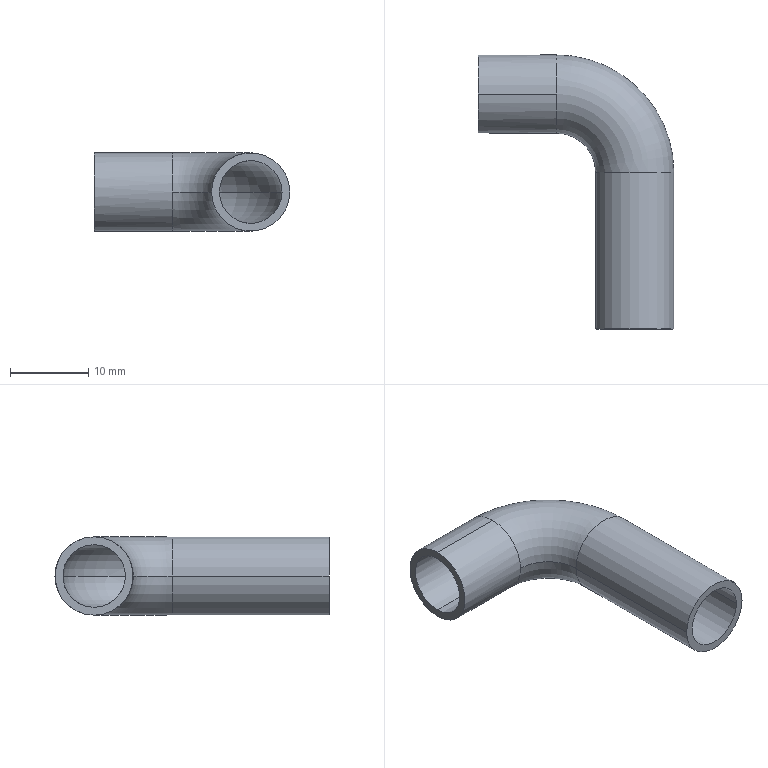Part | SolidWorks | features Sweep 1 | 1 solid | 14 faces | box 25 x 35 x 10 mm | volume 1292 mm3 | cylinder 8 | torus 4 | plane 2 | commonest cylinder face diameters 8 x4 10 x4
STEP:
#1=CARTESIAN_POINT('',(10.,4.,0.));
#2=VERTEX_POINT('',#1);
#3=CARTESIAN_POINT('',(10.,0.,4.));
#4=VERTEX_POINT('',#3);
#5=CARTESIAN_POINT('',(10.,0.,0.));
#6=DIRECTION('',(1.,0.,0.));
#7=DIRECTION('',(0.,0.,-1.));
#8=AXIS2_PLACEMENT_3D('',#5,#6,#7);
#9=CIRCLE('',#8,4.);
#10=EDGE_CURVE('',#2,#4,#9,.T.);
#11=ORIENTED_EDGE('',*,*,#10,.F.);
#12=CARTESIAN_POINT('',(24.,-10.,0.));
#13=VERTEX_POINT('',#12);
#14=CARTESIAN_POINT('',(10.,-10.,0.));
#15=DIRECTION('',(0.,0.,-1.));
#16=DIRECTION('',(-1.,0.,0.));
#17=AXIS2_PLACEMENT_3D('',#14,#15,#16);
#18=CIRCLE('',#17,14.);
#19=EDGE_CURVE('',#2,#13,#18,.T.);
#20=ORIENTED_EDGE('',*,*,#19,.T.);
#21=CARTESIAN_POINT('',(16.,-10.,0.));
#22=VERTEX_POINT('',#21);
#23=CARTESIAN_POINT('',(20.,-10.,0.));
#24=DIRECTION('',(0.,-1.,0.));
#25=DIRECTION('',(0.,0.,-1.));
#26=AXIS2_PLACEMENT_3D('',#23,#24,#25);
#27=CIRCLE('',#26,4.);
#28=EDGE_CURVE('',#13,#22,#27,.T.);
#29=ORIENTED_EDGE('',*,*,#28,.T.);
#30=CARTESIAN_POINT('',(10.,-4.,0.));
#31=VERTEX_POINT('',#30);
#32=CARTESIAN_POINT('',(10.,-10.,0.));
#33=DIRECTION('',(0.,0.,-1.));
#34=DIRECTION('',(-1.,0.,0.));
#35=AXIS2_PLACEMENT_3D('',#32,#33,#34);
#36=CIRCLE('',#35,6.);
#37=EDGE_CURVE('',#31,#22,#36,.T.);
#38=ORIENTED_EDGE('',*,*,#37,.F.);
#39=CARTESIAN_POINT('',(10.,0.,0.));
#40=DIRECTION('',(1.,0.,0.));
#41=DIRECTION('',(0.,0.,-1.));
#42=AXIS2_PLACEMENT_3D('',#39,#40,#41);
#43=CIRCLE('',#42,4.);
#44=EDGE_CURVE('',#4,#31,#43,.T.);
#45=ORIENTED_EDGE('',*,*,#44,.F.);
#46=EDGE_LOOP('',(#11,#20,#29,#38,#45));
#47=FACE_OUTER_BOUND('',#46,.T.);
#48=CARTESIAN_POINT('',(10.,-10.,0.));
#49=DIRECTION('',(0.,0.,-1.));
#50=DIRECTION('',(-1.,0.,0.));
#51=AXIS2_PLACEMENT_3D('',#48,#49,#50);
#52=TOROIDAL_SURFACE('',#51,10.,4.);
#53=ADVANCED_FACE('',(#47),#52,.F.);
#54=CARTESIAN_POINT('',(10.,0.,-5.));
#55=VERTEX_POINT('',#54);
#56=CARTESIAN_POINT('',(10.,5.,0.));
#57=VERTEX_POINT('',#56);
#58=CARTESIAN_POINT('',(10.,0.,0.));
#59=DIRECTION('',(1.,0.,0.));
#60=DIRECTION('',(0.,0.,-1.));
#61=AXIS2_PLACEMENT_3D('',#58,#59,#60);
#62=CIRCLE('',#61,5.);
#63=EDGE_CURVE('',#55,#57,#62,.T.);
#64=ORIENTED_EDGE('',*,*,#63,.T.);
#65=CARTESIAN_POINT('',(25.,-10.,0.));
#66=VERTEX_POINT('',#65);
#67=CARTESIAN_POINT('',(10.,-10.,0.));
#68=DIRECTION('',(0.,0.,-1.));
#69=DIRECTION('',(-1.,0.,0.));
#70=AXIS2_PLACEMENT_3D('',#67,#68,#69);
#71=CIRCLE('',#70,15.);
#72=EDGE_CURVE('',#57,#66,#71,.T.);
#73=ORIENTED_EDGE('',*,*,#72,.T.);
#74=CARTESIAN_POINT('',(15.,-10.,0.));
#75=VERTEX_POINT('',#74);
#76=CARTESIAN_POINT('',(20.,-10.,0.));
#77=DIRECTION('',(0.,-1.,0.));
#78=DIRECTION('',(0.,0.,-1.));
#79=AXIS2_PLACEMENT_3D('',#76,#77,#78);
#80=CIRCLE('',#79,5.);
#81=EDGE_CURVE('',#75,#66,#80,.T.);
#82=ORIENTED_EDGE('',*,*,#81,.F.);
#83=CARTESIAN_POINT('',(10.,-5.,0.));
#84=VERTEX_POINT('',#83);
#85=CARTESIAN_POINT('',(10.,-10.,0.));
#86=DIRECTION('',(0.,0.,-1.));
#87=DIRECTION('',(-1.,0.,0.));
#88=AXIS2_PLACEMENT_3D('',#85,#86,#87);
#89=CIRCLE('',#88,5.);
#90=EDGE_CURVE('',#84,#75,#89,.T.);
#91=ORIENTED_EDGE('',*,*,#90,.F.);
#92=CARTESIAN_POINT('',(10.,0.,0.));
#93=DIRECTION('',(1.,0.,0.));
#94=DIRECTION('',(0.,0.,-1.));
#95=AXIS2_PLACEMENT_3D('',#92,#93,#94);
#96=CIRCLE('',#95,5.);
#97=EDGE_CURVE('',#84,#55,#96,.T.);
#98=ORIENTED_EDGE('',*,*,#97,.T.);
#99=EDGE_LOOP('',(#64,#73,#82,#91,#98));
#100=FACE_OUTER_BOUND('',#99,.T.);
#101=CARTESIAN_POINT('',(10.,-10.,0.));
#102=DIRECTION('',(0.,0.,-1.));
#103=DIRECTION('',(-1.,0.,0.));
#104=AXIS2_PLACEMENT_3D('',#101,#102,#103);
#105=TOROIDAL_SURFACE('',#104,10.,5.);
#106=ADVANCED_FACE('',(#100),#105,.T.);
#107=ORIENTED_EDGE('',*,*,#63,.F.);
#108=CARTESIAN_POINT('',(0.,0.,-5.));
#109=VERTEX_POINT('',#108);
#110=CARTESIAN_POINT('',(10.,0.,-5.));
#111=DIRECTION('',(-1.,0.,0.));
#112=VECTOR('',#111,1000.);
#113=LINE('',#110,#112);
#114=EDGE_CURVE('',#55,#109,#113,.T.);
#115=ORIENTED_EDGE('',*,*,#114,.T.);
#116=CARTESIAN_POINT('',(0.,0.,5.));
#117=VERTEX_POINT('',#116);
#118=CARTESIAN_POINT('',(0.,0.,0.));
#119=DIRECTION('',(1.,0.,0.));
#120=DIRECTION('',(0.,0.,-1.));
#121=AXIS2_PLACEMENT_3D('',#118,#119,#120);
#122=CIRCLE('',#121,5.);
#123=EDGE_CURVE('',#109,#117,#122,.T.);
#124=ORIENTED_EDGE('',*,*,#123,.T.);
#125=CARTESIAN_POINT('',(10.,0.,5.));
#126=VERTEX_POINT('',#125);
#127=CARTESIAN_POINT('',(10.,0.,5.));
#128=DIRECTION('',(-1.,0.,0.));
#129=VECTOR('',#128,1000.);
#130=LINE('',#127,#129);
#131=EDGE_CURVE('',#126,#117,#130,.T.);
#132=ORIENTED_EDGE('',*,*,#131,.F.);
#133=CARTESIAN_POINT('',(10.,0.,0.));
#134=DIRECTION('',(1.,0.,0.));
#135=DIRECTION('',(0.,0.,-1.));
#136=AXIS2_PLACEMENT_3D('',#133,#134,#135);
#137=CIRCLE('',#136,5.);
#138=EDGE_CURVE('',#57,#126,#137,.T.);
#139=ORIENTED_EDGE('',*,*,#138,.F.);
#140=EDGE_LOOP('',(#107,#115,#124,#132,#139));
#141=FACE_OUTER_BOUND('',#140,.T.);
#142=CARTESIAN_POINT('',(10.,0.,0.));
#143=DIRECTION('',(-1.,0.,0.));
#144=DIRECTION('',(0.,0.,1.));
#145=AXIS2_PLACEMENT_3D('',#142,#143,#144);
#146=CYLINDRICAL_SURFACE('',#145,5.);
#147=ADVANCED_FACE('',(#141),#146,.T.);
#148=ORIENTED_EDGE('',*,*,#44,.T.);
#149=CARTESIAN_POINT('',(10.,0.,-4.));
#150=VERTEX_POINT('',#149);
#151=CARTESIAN_POINT('',(10.,0.,0.));
#152=DIRECTION('',(1.,0.,0.));
#153=DIRECTION('',(0.,0.,-1.));
#154=AXIS2_PLACEMENT_3D('',#151,#152,#153);
#155=CIRCLE('',#154,4.);
#156=EDGE_CURVE('',#31,#150,#155,.T.);
#157=ORIENTED_EDGE('',*,*,#156,.T.);
#158=CARTESIAN_POINT('',(0.,0.,-4.));
#159=VERTEX_POINT('',#158);
#160=CARTESIAN_POINT('',(10.,0.,-4.));
#161=DIRECTION('',(-1.,0.,0.));
#162=VECTOR('',#161,1000.);
#163=LINE('',#160,#162);
#164=EDGE_CURVE('',#150,#159,#163,.T.);
#165=ORIENTED_EDGE('',*,*,#164,.T.);
#166=CARTESIAN_POINT('',(0.,0.,4.));
#167=VERTEX_POINT('',#166);
#168=CARTESIAN_POINT('',(0.,0.,0.));
#169=DIRECTION('',(1.,0.,0.));
#170=DIRECTION('',(0.,0.,-1.));
#171=AXIS2_PLACEMENT_3D('',#168,#169,#170);
#172=CIRCLE('',#171,4.);
#173=EDGE_CURVE('',#167,#159,#172,.T.);
#174=ORIENTED_EDGE('',*,*,#173,.F.);
#175=CARTESIAN_POINT('',(10.,0.,4.));
#176=DIRECTION('',(-1.,0.,0.));
#177=VECTOR('',#176,1000.);
#178=LINE('',#175,#177);
#179=EDGE_CURVE('',#4,#167,#178,.T.);
#180=ORIENTED_EDGE('',*,*,#179,.F.);
#181=EDGE_LOOP('',(#148,#157,#165,#174,#180));
#182=FACE_OUTER_BOUND('',#181,.T.);
#183=CARTESIAN_POINT('',(10.,0.,0.));
#184=DIRECTION('',(-1.,0.,0.));
#185=DIRECTION('',(0.,0.,1.));
#186=AXIS2_PLACEMENT_3D('',#183,#184,#185);
#187=CYLINDRICAL_SURFACE('',#186,4.);
#188=ADVANCED_FACE('',(#182),#187,.F.);
#189=CARTESIAN_POINT('',(20.,-10.,0.));
#190=DIRECTION('',(0.,-1.,0.));
#191=DIRECTION('',(0.,0.,-1.));
#192=AXIS2_PLACEMENT_3D('',#189,#190,#191);
#193=CIRCLE('',#192,4.);
#194=EDGE_CURVE('',#22,#13,#193,.T.);
#195=ORIENTED_EDGE('',*,*,#194,.F.);
#196=CARTESIAN_POINT('',(16.,-30.,0.));
#197=VERTEX_POINT('',#196);
#198=CARTESIAN_POINT('',(16.,-10.,0.));
#199=DIRECTION('',(0.,-1.,0.));
#200=VECTOR('',#199,1000.);
#201=LINE('',#198,#200);
#202=EDGE_CURVE('',#22,#197,#201,.T.);
#203=ORIENTED_EDGE('',*,*,#202,.T.);
#204=CARTESIAN_POINT('',(24.,-30.,0.));
#205=VERTEX_POINT('',#204);
#206=CARTESIAN_POINT('',(20.,-30.,0.));
#207=DIRECTION('',(0.,-1.,0.));
#208=DIRECTION('',(0.,0.,-1.));
#209=AXIS2_PLACEMENT_3D('',#206,#207,#208);
#210=CIRCLE('',#209,4.);
#211=EDGE_CURVE('',#197,#205,#210,.T.);
#212=ORIENTED_EDGE('',*,*,#211,.T.);
#213=CARTESIAN_POINT('',(24.,-10.,0.));
#214=DIRECTION('',(0.,-1.,0.));
#215=VECTOR('',#214,1000.);
#216=LINE('',#213,#215);
#217=EDGE_CURVE('',#13,#205,#216,.T.);
#218=ORIENTED_EDGE('',*,*,#217,.F.);
#219=EDGE_LOOP('',(#195,#203,#212,#218));
#220=FACE_OUTER_BOUND('',#219,.T.);
#221=CARTESIAN_POINT('',(20.,-10.,0.));
#222=DIRECTION('',(0.,-1.,0.));
#223=DIRECTION('',(1.,0.,0.));
#224=AXIS2_PLACEMENT_3D('',#221,#222,#223);
#225=CYLINDRICAL_SURFACE('',#224,4.);
#226=ADVANCED_FACE('',(#220),#225,.F.);
#227=CARTESIAN_POINT('',(20.,-10.,0.));
#228=DIRECTION('',(0.,-1.,0.));
#229=DIRECTION('',(0.,0.,-1.));
#230=AXIS2_PLACEMENT_3D('',#227,#228,#229);
#231=CIRCLE('',#230,5.);
#232=EDGE_CURVE('',#66,#75,#231,.T.);
#233=ORIENTED_EDGE('',*,*,#232,.T.);
#234=CARTESIAN_POINT('',(15.,-30.,0.));
#235=VERTEX_POINT('',#234);
#236=CARTESIAN_POINT('',(15.,-10.,0.));
#237=DIRECTION('',(0.,-1.,0.));
#238=VECTOR('',#237,1000.);
#239=LINE('',#236,#238);
#240=EDGE_CURVE('',#75,#235,#239,.T.);
#241=ORIENTED_EDGE('',*,*,#240,.T.);
#242=CARTESIAN_POINT('',(25.,-30.,0.));
#243=VERTEX_POINT('',#242);
#244=CARTESIAN_POINT('',(20.,-30.,0.));
#245=DIRECTION('',(0.,-1.,0.));
#246=DIRECTION('',(0.,0.,-1.));
#247=AXIS2_PLACEMENT_3D('',#244,#245,#246);
#248=CIRCLE('',#247,5.);
#249=EDGE_CURVE('',#243,#235,#248,.T.);
#250=ORIENTED_EDGE('',*,*,#249,.F.);
#251=CARTESIAN_POINT('',(25.,-10.,0.));
#252=DIRECTION('',(0.,-1.,0.));
#253=VECTOR('',#252,1000.);
#254=LINE('',#251,#253);
#255=EDGE_CURVE('',#66,#243,#254,.T.);
#256=ORIENTED_EDGE('',*,*,#255,.F.);
#257=EDGE_LOOP('',(#233,#241,#250,#256));
#258=FACE_OUTER_BOUND('',#257,.T.);
#259=CARTESIAN_POINT('',(20.,-10.,0.));
#260=DIRECTION('',(0.,-1.,0.));
#261=DIRECTION('',(1.,0.,0.));
#262=AXIS2_PLACEMENT_3D('',#259,#260,#261);
#263=CYLINDRICAL_SURFACE('',#262,5.);
#264=ADVANCED_FACE('',(#258),#263,.T.);
#265=ORIENTED_EDGE('',*,*,#240,.F.);
#266=ORIENTED_EDGE('',*,*,#81,.T.);
#267=ORIENTED_EDGE('',*,*,#255,.T.);
#268=CARTESIAN_POINT('',(20.,-30.,0.));
#269=DIRECTION('',(0.,-1.,0.));
#270=DIRECTION('',(0.,0.,-1.));
#271=AXIS2_PLACEMENT_3D('',#268,#269,#270);
#272=CIRCLE('',#271,5.);
#273=EDGE_CURVE('',#235,#243,#272,.T.);
#274=ORIENTED_EDGE('',*,*,#273,.F.);
#275=EDGE_LOOP('',(#265,#266,#267,#274));
#276=FACE_OUTER_BOUND('',#275,.T.);
#277=CARTESIAN_POINT('',(20.,-10.,0.));
#278=DIRECTION('',(0.,-1.,0.));
#279=DIRECTION('',(1.,0.,0.));
#280=AXIS2_PLACEMENT_3D('',#277,#278,#279);
#281=CYLINDRICAL_SURFACE('',#280,5.);
#282=ADVANCED_FACE('',(#276),#281,.T.);
#283=ORIENTED_EDGE('',*,*,#202,.F.);
#284=ORIENTED_EDGE('',*,*,#28,.F.);
#285=ORIENTED_EDGE('',*,*,#217,.T.);
#286=CARTESIAN_POINT('',(20.,-30.,0.));
#287=DIRECTION('',(0.,-1.,0.));
#288=DIRECTION('',(0.,0.,-1.));
#289=AXIS2_PLACEMENT_3D('',#286,#287,#288);
#290=CIRCLE('',#289,4.);
#291=EDGE_CURVE('',#205,#197,#290,.T.);
#292=ORIENTED_EDGE('',*,*,#291,.T.);
#293=EDGE_LOOP('',(#283,#284,#285,#292));
#294=FACE_OUTER_BOUND('',#293,.T.);
#295=CARTESIAN_POINT('',(20.,-10.,0.));
#296=DIRECTION('',(0.,-1.,0.));
#297=DIRECTION('',(1.,0.,0.));
#298=AXIS2_PLACEMENT_3D('',#295,#296,#297);
#299=CYLINDRICAL_SURFACE('',#298,4.);
#300=ADVANCED_FACE('',(#294),#299,.F.);
#301=ORIENTED_EDGE('',*,*,#72,.F.);
#302=ORIENTED_EDGE('',*,*,#138,.T.);
#303=CARTESIAN_POINT('',(10.,0.,0.));
#304=DIRECTION('',(1.,0.,0.));
#305=DIRECTION('',(0.,0.,-1.));
#306=AXIS2_PLACEMENT_3D('',#303,#304,#305);
#307=CIRCLE('',#306,5.);
#308=EDGE_CURVE('',#126,#84,#307,.T.);
#309=ORIENTED_EDGE('',*,*,#308,.T.);
#310=ORIENTED_EDGE('',*,*,#90,.T.);
#311=ORIENTED_EDGE('',*,*,#232,.F.);
#312=EDGE_LOOP('',(#301,#302,#309,#310,#311));
#313=FACE_OUTER_BOUND('',#312,.T.);
#314=CARTESIAN_POINT('',(10.,-10.,0.));
#315=DIRECTION('',(0.,0.,-1.));
#316=DIRECTION('',(-1.,0.,0.));
#317=AXIS2_PLACEMENT_3D('',#314,#315,#316);
#318=TOROIDAL_SURFACE('',#317,10.,5.);
#319=ADVANCED_FACE('',(#313),#318,.T.);
#320=ORIENTED_EDGE('',*,*,#19,.F.);
#321=CARTESIAN_POINT('',(10.,0.,0.));
#322=DIRECTION('',(1.,0.,0.));
#323=DIRECTION('',(0.,0.,-1.));
#324=AXIS2_PLACEMENT_3D('',#321,#322,#323);
#325=CIRCLE('',#324,4.);
#326=EDGE_CURVE('',#150,#2,#325,.T.);
#327=ORIENTED_EDGE('',*,*,#326,.F.);
#328=ORIENTED_EDGE('',*,*,#156,.F.);
#329=ORIENTED_EDGE('',*,*,#37,.T.);
#330=ORIENTED_EDGE('',*,*,#194,.T.);
#331=EDGE_LOOP('',(#320,#327,#328,#329,#330));
#332=FACE_OUTER_BOUND('',#331,.T.);
#333=CARTESIAN_POINT('',(10.,-10.,0.));
#334=DIRECTION('',(0.,0.,-1.));
#335=DIRECTION('',(-1.,0.,0.));
#336=AXIS2_PLACEMENT_3D('',#333,#334,#335);
#337=TOROIDAL_SURFACE('',#336,10.,4.);
#338=ADVANCED_FACE('',(#332),#337,.F.);
#339=ORIENTED_EDGE('',*,*,#164,.F.);
#340=ORIENTED_EDGE('',*,*,#326,.T.);
#341=ORIENTED_EDGE('',*,*,#10,.T.);
#342=ORIENTED_EDGE('',*,*,#179,.T.);
#343=CARTESIAN_POINT('',(0.,0.,0.));
#344=DIRECTION('',(1.,0.,0.));
#345=DIRECTION('',(0.,0.,-1.));
#346=AXIS2_PLACEMENT_3D('',#343,#344,#345);
#347=CIRCLE('',#346,4.);
#348=EDGE_CURVE('',#159,#167,#347,.T.);
#349=ORIENTED_EDGE('',*,*,#348,.F.);
#350=EDGE_LOOP('',(#339,#340,#341,#342,#349));
#351=FACE_OUTER_BOUND('',#350,.T.);
#352=CARTESIAN_POINT('',(10.,0.,0.));
#353=DIRECTION('',(-1.,0.,0.));
#354=DIRECTION('',(0.,0.,1.));
#355=AXIS2_PLACEMENT_3D('',#352,#353,#354);
#356=CYLINDRICAL_SURFACE('',#355,4.);
#357=ADVANCED_FACE('',(#351),#356,.F.);
#358=ORIENTED_EDGE('',*,*,#114,.F.);
#359=ORIENTED_EDGE('',*,*,#97,.F.);
#360=ORIENTED_EDGE('',*,*,#308,.F.);
#361=ORIENTED_EDGE('',*,*,#131,.T.);
#362=CARTESIAN_POINT('',(0.,0.,0.));
#363=DIRECTION('',(1.,0.,0.));
#364=DIRECTION('',(0.,0.,-1.));
#365=AXIS2_PLACEMENT_3D('',#362,#363,#364);
#366=CIRCLE('',#365,5.);
#367=EDGE_CURVE('',#117,#109,#366,.T.);
#368=ORIENTED_EDGE('',*,*,#367,.T.);
#369=EDGE_LOOP('',(#358,#359,#360,#361,#368));
#370=FACE_OUTER_BOUND('',#369,.T.);
#371=CARTESIAN_POINT('',(10.,0.,0.));
#372=DIRECTION('',(-1.,0.,0.));
#373=DIRECTION('',(0.,0.,1.));
#374=AXIS2_PLACEMENT_3D('',#371,#372,#373);
#375=CYLINDRICAL_SURFACE('',#374,5.);
#376=ADVANCED_FACE('',(#370),#375,.T.);
#377=ORIENTED_EDGE('',*,*,#291,.F.);
#378=ORIENTED_EDGE('',*,*,#211,.F.);
#379=EDGE_LOOP('',(#377,#378));
#380=FACE_BOUND('',#379,.T.);
#381=ORIENTED_EDGE('',*,*,#249,.T.);
#382=ORIENTED_EDGE('',*,*,#273,.T.);
#383=EDGE_LOOP('',(#381,#382));
#384=FACE_OUTER_BOUND('',#383,.T.);
#385=CARTESIAN_POINT('',(20.,-30.,0.));
#386=DIRECTION('',(0.,-1.,0.));
#387=DIRECTION('',(0.,0.,-1.));
#388=AXIS2_PLACEMENT_3D('',#385,#386,#387);
#389=PLANE('',#388);
#390=ADVANCED_FACE('',(#380,#384),#389,.T.);
#391=ORIENTED_EDGE('',*,*,#173,.T.);
#392=ORIENTED_EDGE('',*,*,#348,.T.);
#393=EDGE_LOOP('',(#391,#392));
#394=FACE_BOUND('',#393,.T.);
#395=ORIENTED_EDGE('',*,*,#367,.F.);
#396=ORIENTED_EDGE('',*,*,#123,.F.);
#397=EDGE_LOOP('',(#395,#396));
#398=FACE_OUTER_BOUND('',#397,.T.);
#399=CARTESIAN_POINT('',(0.,0.,0.));
#400=DIRECTION('',(1.,0.,0.));
#401=DIRECTION('',(0.,0.,-1.));
#402=AXIS2_PLACEMENT_3D('',#399,#400,#401);
#403=PLANE('',#402);
#404=ADVANCED_FACE('',(#394,#398),#403,.F.);
#405=CLOSED_SHELL('',(#53,#106,#147,#188,#226,#264,#282,#300,#319,#338,#357,#376,#390,#404));
#406=MANIFOLD_SOLID_BREP('',#405);
#407=CARTESIAN_POINT('',(0.,0.,0.));
#408=DIRECTION('',(0.,0.,1.));
#409=DIRECTION('',(1.,0.,0.));
#410=AXIS2_PLACEMENT_3D('',#407,#408,#409);
#411=(LENGTH_UNIT()NAMED_UNIT(*)SI_UNIT(.MILLI.,.METRE.));
#412=UNCERTAINTY_MEASURE_WITH_UNIT(LENGTH_MEASURE(0.00001),#411,'','');
#413=(NAMED_UNIT(*)PLANE_ANGLE_UNIT()SI_UNIT($,.RADIAN.));
#414=(NAMED_UNIT(*)SI_UNIT($,.STERADIAN.)SOLID_ANGLE_UNIT());
#415=(GEOMETRIC_REPRESENTATION_CONTEXT(3)GLOBAL_UNCERTAINTY_ASSIGNED_CONTEXT((#412))GLOBAL_UNIT_ASSIGNED_CONTEXT((#411,#413,#414))REPRESENTATION_CONTEXT('',''));
#416=ADVANCED_BREP_SHAPE_REPRESENTATION('',(#406,#410),#415);